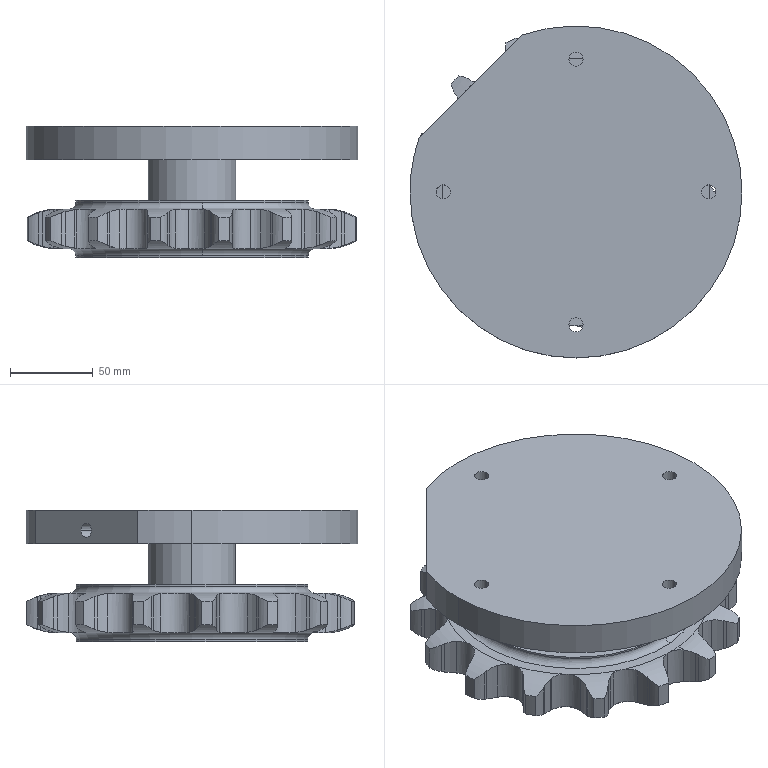Part | SolidWorks | 4 solids | 261 faces | box 200 x 200 x 79.02 mm | volume 1384453 mm3 | cylinder 152 | plane 55 | torus 52 | cone 2 | commonest cylinder face diameters 32.838 x32 58.009 x31 22.441 x19 199 x15 8.5 x10 50 x8